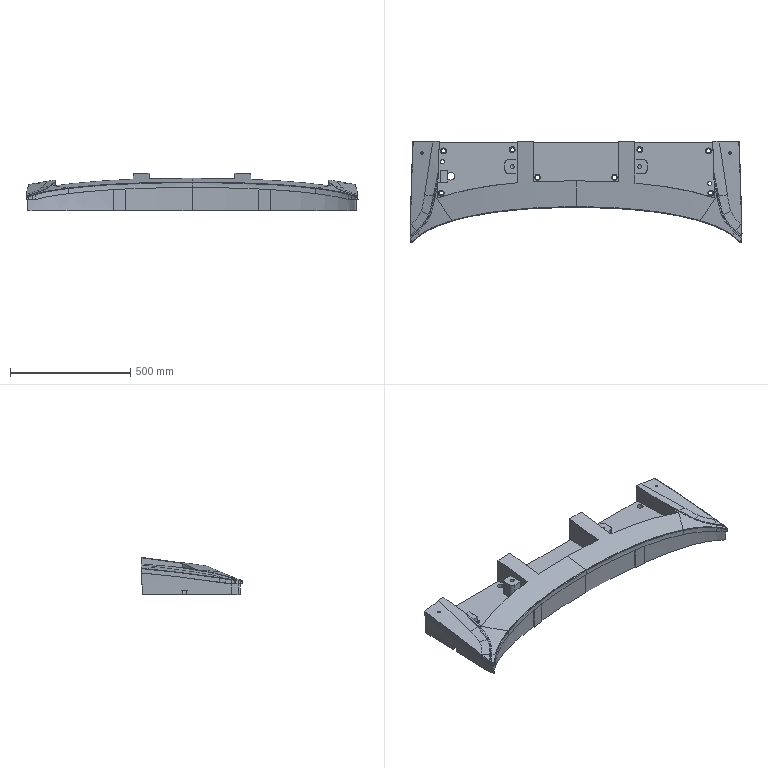Part | NX | features solid 2 | 1 solid | 252 faces | box 1379 x 421.453 x 154.469 mm | volume 34149889 mm3 | spline 147 | plane 67 | cylinder 36 | cone 2 | commonest cylinder face diameters 25 x17 17 x8 16 x4 30 x4 10 x2 32 x1